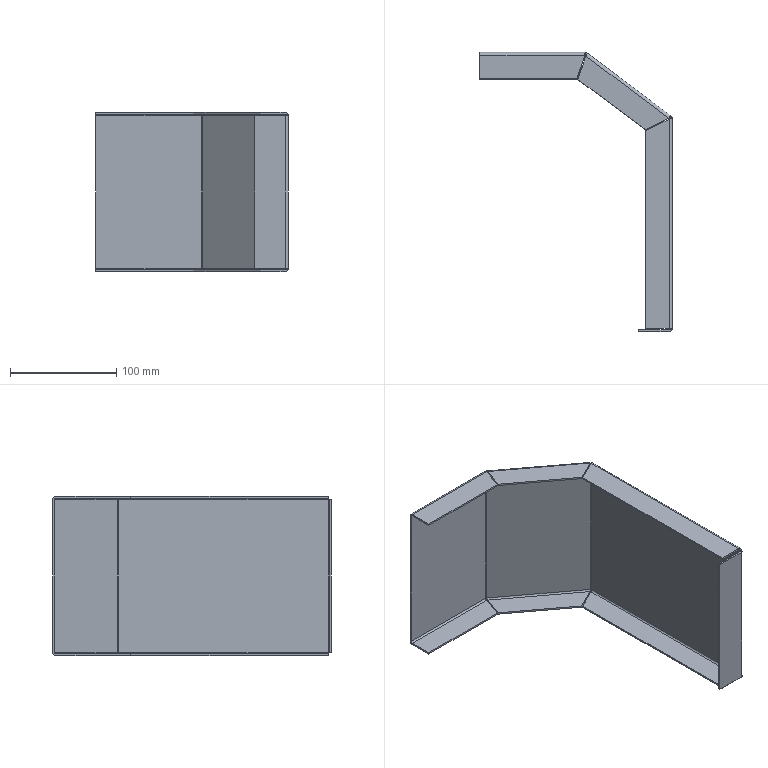Part | STEP file | 1 solid | 78 faces | box 181.5 x 263 x 150 mm | volume 122189 mm3 | plane 52 | cylinder 18 | spline 8 | commonest cylinder face diameters 3 x9 6 x9